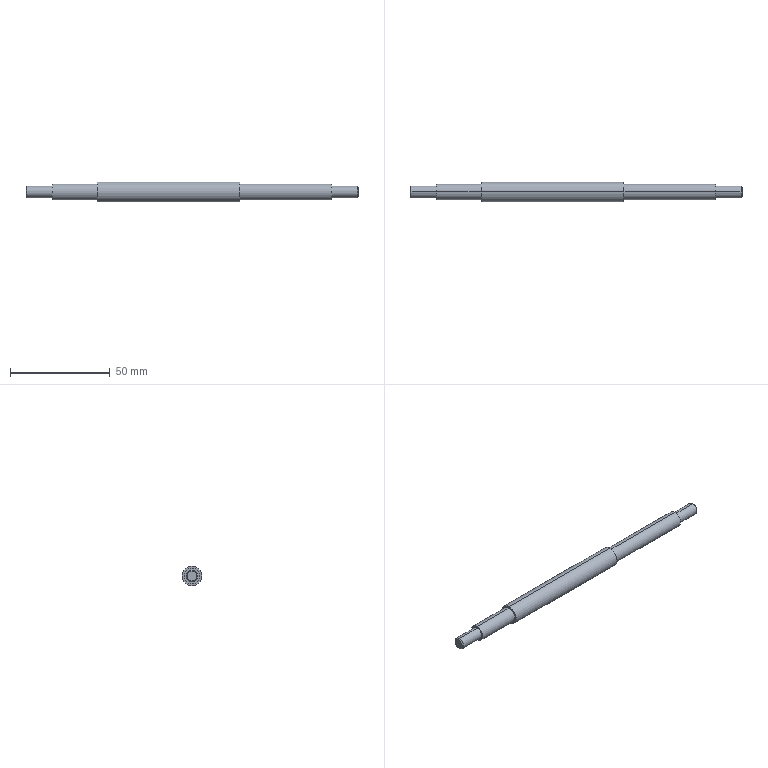Part | SolidWorks | features Revolution 1 | 1 solid | 20 faces | box 166.354 x 10 x 10 mm | volume 9800 mm3 | cylinder 10 | plane 6 | cone 4 | commonest cylinder face diameters 6 x4 8 x4 10 x2
STEP:
#1=CARTESIAN_POINT('',(-205.748,-31.205,-3.));
#2=VERTEX_POINT('',#1);
#3=CARTESIAN_POINT('',(-205.748,-31.205,3.));
#4=VERTEX_POINT('',#3);
#5=CARTESIAN_POINT('',(-205.748,-31.205,0.));
#6=DIRECTION('',(1.,0.,0.));
#7=DIRECTION('',(0.,0.,-1.));
#8=AXIS2_PLACEMENT_3D('',#5,#6,#7);
#9=CIRCLE('',#8,3.);
#10=EDGE_CURVE('',#2,#4,#9,.T.);
#11=ORIENTED_EDGE('',*,*,#10,.T.);
#12=CARTESIAN_POINT('',(-193.072,-31.205,3.));
#13=VERTEX_POINT('',#12);
#14=CARTESIAN_POINT('',(-206.248,-31.205,3.));
#15=DIRECTION('',(1.,0.,0.));
#16=VECTOR('',#15,1000.);
#17=LINE('',#14,#16);
#18=EDGE_CURVE('',#4,#13,#17,.T.);
#19=ORIENTED_EDGE('',*,*,#18,.T.);
#20=CARTESIAN_POINT('',(-193.072,-31.205,-3.));
#21=VERTEX_POINT('',#20);
#22=CARTESIAN_POINT('',(-193.072,-31.205,0.));
#23=DIRECTION('',(1.,0.,0.));
#24=DIRECTION('',(0.,0.,-1.));
#25=AXIS2_PLACEMENT_3D('',#22,#23,#24);
#26=CIRCLE('',#25,3.);
#27=EDGE_CURVE('',#21,#13,#26,.T.);
#28=ORIENTED_EDGE('',*,*,#27,.F.);
#29=CARTESIAN_POINT('',(-206.248,-31.205,-3.));
#30=DIRECTION('',(1.,0.,0.));
#31=VECTOR('',#30,1000.);
#32=LINE('',#29,#31);
#33=EDGE_CURVE('',#2,#21,#32,.T.);
#34=ORIENTED_EDGE('',*,*,#33,.F.);
#35=EDGE_LOOP('',(#11,#19,#28,#34));
#36=FACE_OUTER_BOUND('',#35,.T.);
#37=CARTESIAN_POINT('',(-206.248,-31.205,0.));
#38=DIRECTION('',(1.,0.,0.));
#39=DIRECTION('',(0.,0.,-1.));
#40=AXIS2_PLACEMENT_3D('',#37,#38,#39);
#41=CYLINDRICAL_SURFACE('',#40,3.);
#42=ADVANCED_FACE('',(#36),#41,.T.);
#43=CARTESIAN_POINT('',(-206.248,-31.205,-2.5));
#44=VERTEX_POINT('',#43);
#45=CARTESIAN_POINT('',(-206.248,-31.205,2.5));
#46=VERTEX_POINT('',#45);
#47=CARTESIAN_POINT('',(-206.248,-31.205,0.));
#48=DIRECTION('',(1.,0.,0.));
#49=DIRECTION('',(0.,0.,-1.));
#50=AXIS2_PLACEMENT_3D('',#47,#48,#49);
#51=CIRCLE('',#50,2.5);
#52=EDGE_CURVE('',#44,#46,#51,.T.);
#53=ORIENTED_EDGE('',*,*,#52,.T.);
#54=CARTESIAN_POINT('',(-205.748,-31.205,3.));
#55=DIRECTION('',(0.7071,0.,0.7071));
#56=VECTOR('',#55,1000.);
#57=LINE('',#54,#56);
#58=EDGE_CURVE('',#46,#4,#57,.T.);
#59=ORIENTED_EDGE('',*,*,#58,.T.);
#60=ORIENTED_EDGE('',*,*,#10,.F.);
#61=CARTESIAN_POINT('',(-205.748,-31.205,-3.));
#62=DIRECTION('',(0.7071,0.,-0.7071));
#63=VECTOR('',#62,1000.);
#64=LINE('',#61,#63);
#65=EDGE_CURVE('',#44,#2,#64,.T.);
#66=ORIENTED_EDGE('',*,*,#65,.F.);
#67=EDGE_LOOP('',(#53,#59,#60,#66));
#68=FACE_OUTER_BOUND('',#67,.T.);
#69=CARTESIAN_POINT('',(-205.748,-31.205,0.));
#70=DIRECTION('',(1.,0.,0.));
#71=DIRECTION('',(0.,0.,-1.));
#72=AXIS2_PLACEMENT_3D('',#69,#70,#71);
#73=CONICAL_SURFACE('',#72,3.,0.7854);
#74=ADVANCED_FACE('',(#68),#73,.T.);
#75=CARTESIAN_POINT('',(-39.895,-31.205,-2.5));
#76=VERTEX_POINT('',#75);
#77=CARTESIAN_POINT('',(-39.895,-31.205,2.5));
#78=VERTEX_POINT('',#77);
#79=CARTESIAN_POINT('',(-39.895,-31.205,0.));
#80=DIRECTION('',(1.,0.,0.));
#81=DIRECTION('',(0.,0.,-1.));
#82=AXIS2_PLACEMENT_3D('',#79,#80,#81);
#83=CIRCLE('',#82,2.5);
#84=EDGE_CURVE('',#76,#78,#83,.T.);
#85=ORIENTED_EDGE('',*,*,#84,.F.);
#86=CARTESIAN_POINT('',(-40.395,-31.205,-3.));
#87=VERTEX_POINT('',#86);
#88=CARTESIAN_POINT('',(-39.895,-31.205,-2.5));
#89=DIRECTION('',(-0.7071,0.,-0.7071));
#90=VECTOR('',#89,1000.);
#91=LINE('',#88,#90);
#92=EDGE_CURVE('',#76,#87,#91,.T.);
#93=ORIENTED_EDGE('',*,*,#92,.T.);
#94=CARTESIAN_POINT('',(-40.395,-31.205,3.));
#95=VERTEX_POINT('',#94);
#96=CARTESIAN_POINT('',(-40.395,-31.205,0.));
#97=DIRECTION('',(1.,0.,0.));
#98=DIRECTION('',(0.,0.,-1.));
#99=AXIS2_PLACEMENT_3D('',#96,#97,#98);
#100=CIRCLE('',#99,3.);
#101=EDGE_CURVE('',#87,#95,#100,.T.);
#102=ORIENTED_EDGE('',*,*,#101,.T.);
#103=CARTESIAN_POINT('',(-39.895,-31.205,2.5));
#104=DIRECTION('',(-0.7071,0.,0.7071));
#105=VECTOR('',#104,1000.);
#106=LINE('',#103,#105);
#107=EDGE_CURVE('',#78,#95,#106,.T.);
#108=ORIENTED_EDGE('',*,*,#107,.F.);
#109=EDGE_LOOP('',(#85,#93,#102,#108));
#110=FACE_OUTER_BOUND('',#109,.T.);
#111=CARTESIAN_POINT('',(-39.895,-31.205,0.));
#112=DIRECTION('',(-1.,0.,0.));
#113=DIRECTION('',(0.,0.,1.));
#114=AXIS2_PLACEMENT_3D('',#111,#112,#113);
#115=CONICAL_SURFACE('',#114,2.5,0.7854);
#116=ADVANCED_FACE('',(#110),#115,.T.);
#117=CARTESIAN_POINT('',(-53.072,-31.205,-3.));
#118=VERTEX_POINT('',#117);
#119=CARTESIAN_POINT('',(-53.072,-31.205,3.));
#120=VERTEX_POINT('',#119);
#121=CARTESIAN_POINT('',(-53.072,-31.205,0.));
#122=DIRECTION('',(1.,0.,0.));
#123=DIRECTION('',(0.,0.,-1.));
#124=AXIS2_PLACEMENT_3D('',#121,#122,#123);
#125=CIRCLE('',#124,3.);
#126=EDGE_CURVE('',#118,#120,#125,.T.);
#127=ORIENTED_EDGE('',*,*,#126,.T.);
#128=CARTESIAN_POINT('',(-206.248,-31.205,3.));
#129=DIRECTION('',(1.,0.,0.));
#130=VECTOR('',#129,1000.);
#131=LINE('',#128,#130);
#132=EDGE_CURVE('',#120,#95,#131,.T.);
#133=ORIENTED_EDGE('',*,*,#132,.T.);
#134=ORIENTED_EDGE('',*,*,#101,.F.);
#135=CARTESIAN_POINT('',(-206.248,-31.205,-3.));
#136=DIRECTION('',(1.,0.,0.));
#137=VECTOR('',#136,1000.);
#138=LINE('',#135,#137);
#139=EDGE_CURVE('',#118,#87,#138,.T.);
#140=ORIENTED_EDGE('',*,*,#139,.F.);
#141=EDGE_LOOP('',(#127,#133,#134,#140));
#142=FACE_OUTER_BOUND('',#141,.T.);
#143=CARTESIAN_POINT('',(-206.248,-31.205,0.));
#144=DIRECTION('',(1.,0.,0.));
#145=DIRECTION('',(0.,0.,-1.));
#146=AXIS2_PLACEMENT_3D('',#143,#144,#145);
#147=CYLINDRICAL_SURFACE('',#146,3.);
#148=ADVANCED_FACE('',(#142),#147,.T.);
#149=CARTESIAN_POINT('',(-99.022,-31.205,-4.));
#150=VERTEX_POINT('',#149);
#151=CARTESIAN_POINT('',(-99.022,-31.205,4.));
#152=VERTEX_POINT('',#151);
#153=CARTESIAN_POINT('',(-99.022,-31.205,0.));
#154=DIRECTION('',(1.,0.,0.));
#155=DIRECTION('',(0.,0.,-1.));
#156=AXIS2_PLACEMENT_3D('',#153,#154,#155);
#157=CIRCLE('',#156,4.);
#158=EDGE_CURVE('',#150,#152,#157,.T.);
#159=ORIENTED_EDGE('',*,*,#158,.T.);
#160=CARTESIAN_POINT('',(-53.072,-31.205,4.));
#161=VERTEX_POINT('',#160);
#162=CARTESIAN_POINT('',(-206.248,-31.205,4.));
#163=DIRECTION('',(1.,0.,0.));
#164=VECTOR('',#163,1000.);
#165=LINE('',#162,#164);
#166=EDGE_CURVE('',#152,#161,#165,.T.);
#167=ORIENTED_EDGE('',*,*,#166,.T.);
#168=CARTESIAN_POINT('',(-53.072,-31.205,-4.));
#169=VERTEX_POINT('',#168);
#170=CARTESIAN_POINT('',(-53.072,-31.205,0.));
#171=DIRECTION('',(1.,0.,0.));
#172=DIRECTION('',(0.,0.,-1.));
#173=AXIS2_PLACEMENT_3D('',#170,#171,#172);
#174=CIRCLE('',#173,4.);
#175=EDGE_CURVE('',#169,#161,#174,.T.);
#176=ORIENTED_EDGE('',*,*,#175,.F.);
#177=CARTESIAN_POINT('',(-206.248,-31.205,-4.));
#178=DIRECTION('',(1.,0.,0.));
#179=VECTOR('',#178,1000.);
#180=LINE('',#177,#179);
#181=EDGE_CURVE('',#150,#169,#180,.T.);
#182=ORIENTED_EDGE('',*,*,#181,.F.);
#183=EDGE_LOOP('',(#159,#167,#176,#182));
#184=FACE_OUTER_BOUND('',#183,.T.);
#185=CARTESIAN_POINT('',(-206.248,-31.205,0.));
#186=DIRECTION('',(1.,0.,0.));
#187=DIRECTION('',(0.,0.,-1.));
#188=AXIS2_PLACEMENT_3D('',#185,#186,#187);
#189=CYLINDRICAL_SURFACE('',#188,4.);
#190=ADVANCED_FACE('',(#184),#189,.T.);
#191=CARTESIAN_POINT('',(-170.527,-31.205,-5.));
#192=VERTEX_POINT('',#191);
#193=CARTESIAN_POINT('',(-170.527,-31.205,5.));
#194=VERTEX_POINT('',#193);
#195=CARTESIAN_POINT('',(-170.527,-31.205,0.));
#196=DIRECTION('',(1.,0.,0.));
#197=DIRECTION('',(0.,0.,-1.));
#198=AXIS2_PLACEMENT_3D('',#195,#196,#197);
#199=CIRCLE('',#198,5.);
#200=EDGE_CURVE('',#192,#194,#199,.T.);
#201=ORIENTED_EDGE('',*,*,#200,.T.);
#202=CARTESIAN_POINT('',(-99.022,-31.205,5.));
#203=VERTEX_POINT('',#202);
#204=CARTESIAN_POINT('',(-206.248,-31.205,5.));
#205=DIRECTION('',(1.,0.,0.));
#206=VECTOR('',#205,1000.);
#207=LINE('',#204,#206);
#208=EDGE_CURVE('',#194,#203,#207,.T.);
#209=ORIENTED_EDGE('',*,*,#208,.T.);
#210=CARTESIAN_POINT('',(-99.022,-31.205,-5.));
#211=VERTEX_POINT('',#210);
#212=CARTESIAN_POINT('',(-99.022,-31.205,0.));
#213=DIRECTION('',(1.,0.,0.));
#214=DIRECTION('',(0.,0.,-1.));
#215=AXIS2_PLACEMENT_3D('',#212,#213,#214);
#216=CIRCLE('',#215,5.);
#217=EDGE_CURVE('',#211,#203,#216,.T.);
#218=ORIENTED_EDGE('',*,*,#217,.F.);
#219=CARTESIAN_POINT('',(-206.248,-31.205,-5.));
#220=DIRECTION('',(1.,0.,0.));
#221=VECTOR('',#220,1000.);
#222=LINE('',#219,#221);
#223=EDGE_CURVE('',#192,#211,#222,.T.);
#224=ORIENTED_EDGE('',*,*,#223,.F.);
#225=EDGE_LOOP('',(#201,#209,#218,#224));
#226=FACE_OUTER_BOUND('',#225,.T.);
#227=CARTESIAN_POINT('',(-206.248,-31.205,0.));
#228=DIRECTION('',(1.,0.,0.));
#229=DIRECTION('',(0.,0.,-1.));
#230=AXIS2_PLACEMENT_3D('',#227,#228,#229);
#231=CYLINDRICAL_SURFACE('',#230,5.);
#232=ADVANCED_FACE('',(#226),#231,.T.);
#233=CARTESIAN_POINT('',(-193.072,-31.205,-4.));
#234=VERTEX_POINT('',#233);
#235=CARTESIAN_POINT('',(-193.072,-31.205,4.));
#236=VERTEX_POINT('',#235);
#237=CARTESIAN_POINT('',(-193.072,-31.205,0.));
#238=DIRECTION('',(1.,0.,0.));
#239=DIRECTION('',(0.,0.,-1.));
#240=AXIS2_PLACEMENT_3D('',#237,#238,#239);
#241=CIRCLE('',#240,4.);
#242=EDGE_CURVE('',#234,#236,#241,.T.);
#243=ORIENTED_EDGE('',*,*,#242,.T.);
#244=CARTESIAN_POINT('',(-170.527,-31.205,4.));
#245=VERTEX_POINT('',#244);
#246=CARTESIAN_POINT('',(-206.248,-31.205,4.));
#247=DIRECTION('',(1.,0.,0.));
#248=VECTOR('',#247,1000.);
#249=LINE('',#246,#248);
#250=EDGE_CURVE('',#236,#245,#249,.T.);
#251=ORIENTED_EDGE('',*,*,#250,.T.);
#252=CARTESIAN_POINT('',(-170.527,-31.205,-4.));
#253=VERTEX_POINT('',#252);
#254=CARTESIAN_POINT('',(-170.527,-31.205,0.));
#255=DIRECTION('',(1.,0.,0.));
#256=DIRECTION('',(0.,0.,-1.));
#257=AXIS2_PLACEMENT_3D('',#254,#255,#256);
#258=CIRCLE('',#257,4.);
#259=EDGE_CURVE('',#253,#245,#258,.T.);
#260=ORIENTED_EDGE('',*,*,#259,.F.);
#261=CARTESIAN_POINT('',(-206.248,-31.205,-4.));
#262=DIRECTION('',(1.,0.,0.));
#263=VECTOR('',#262,1000.);
#264=LINE('',#261,#263);
#265=EDGE_CURVE('',#234,#253,#264,.T.);
#266=ORIENTED_EDGE('',*,*,#265,.F.);
#267=EDGE_LOOP('',(#243,#251,#260,#266));
#268=FACE_OUTER_BOUND('',#267,.T.);
#269=CARTESIAN_POINT('',(-206.248,-31.205,0.));
#270=DIRECTION('',(1.,0.,0.));
#271=DIRECTION('',(0.,0.,-1.));
#272=AXIS2_PLACEMENT_3D('',#269,#270,#271);
#273=CYLINDRICAL_SURFACE('',#272,4.);
#274=ADVANCED_FACE('',(#268),#273,.T.);
#275=ORIENTED_EDGE('',*,*,#250,.F.);
#276=CARTESIAN_POINT('',(-193.072,-31.205,0.));
#277=DIRECTION('',(1.,0.,0.));
#278=DIRECTION('',(0.,0.,-1.));
#279=AXIS2_PLACEMENT_3D('',#276,#277,#278);
#280=CIRCLE('',#279,4.);
#281=EDGE_CURVE('',#236,#234,#280,.T.);
#282=ORIENTED_EDGE('',*,*,#281,.T.);
#283=ORIENTED_EDGE('',*,*,#265,.T.);
#284=CARTESIAN_POINT('',(-170.527,-31.205,0.));
#285=DIRECTION('',(1.,0.,0.));
#286=DIRECTION('',(0.,0.,-1.));
#287=AXIS2_PLACEMENT_3D('',#284,#285,#286);
#288=CIRCLE('',#287,4.);
#289=EDGE_CURVE('',#245,#253,#288,.T.);
#290=ORIENTED_EDGE('',*,*,#289,.F.);
#291=EDGE_LOOP('',(#275,#282,#283,#290));
#292=FACE_OUTER_BOUND('',#291,.T.);
#293=CARTESIAN_POINT('',(-206.248,-31.205,0.));
#294=DIRECTION('',(1.,0.,0.));
#295=DIRECTION('',(0.,0.,-1.));
#296=AXIS2_PLACEMENT_3D('',#293,#294,#295);
#297=CYLINDRICAL_SURFACE('',#296,4.);
#298=ADVANCED_FACE('',(#292),#297,.T.);
#299=ORIENTED_EDGE('',*,*,#259,.T.);
#300=ORIENTED_EDGE('',*,*,#289,.T.);
#301=EDGE_LOOP('',(#299,#300));
#302=FACE_BOUND('',#301,.T.);
#303=ORIENTED_EDGE('',*,*,#200,.F.);
#304=CARTESIAN_POINT('',(-170.527,-31.205,0.));
#305=DIRECTION('',(1.,0.,0.));
#306=DIRECTION('',(0.,0.,-1.));
#307=AXIS2_PLACEMENT_3D('',#304,#305,#306);
#308=CIRCLE('',#307,5.);
#309=EDGE_CURVE('',#194,#192,#308,.T.);
#310=ORIENTED_EDGE('',*,*,#309,.F.);
#311=EDGE_LOOP('',(#303,#310));
#312=FACE_OUTER_BOUND('',#311,.T.);
#313=CARTESIAN_POINT('',(-170.527,-27.205,0.));
#314=DIRECTION('',(-1.,0.,0.));
#315=DIRECTION('',(0.,0.,1.));
#316=AXIS2_PLACEMENT_3D('',#313,#314,#315);
#317=PLANE('',#316);
#318=ADVANCED_FACE('',(#302,#312),#317,.T.);
#319=ORIENTED_EDGE('',*,*,#208,.F.);
#320=ORIENTED_EDGE('',*,*,#309,.T.);
#321=ORIENTED_EDGE('',*,*,#223,.T.);
#322=CARTESIAN_POINT('',(-99.022,-31.205,0.));
#323=DIRECTION('',(1.,0.,0.));
#324=DIRECTION('',(0.,0.,-1.));
#325=AXIS2_PLACEMENT_3D('',#322,#323,#324);
#326=CIRCLE('',#325,5.);
#327=EDGE_CURVE('',#203,#211,#326,.T.);
#328=ORIENTED_EDGE('',*,*,#327,.F.);
#329=EDGE_LOOP('',(#319,#320,#321,#328));
#330=FACE_OUTER_BOUND('',#329,.T.);
#331=CARTESIAN_POINT('',(-206.248,-31.205,0.));
#332=DIRECTION('',(1.,0.,0.));
#333=DIRECTION('',(0.,0.,-1.));
#334=AXIS2_PLACEMENT_3D('',#331,#332,#333);
#335=CYLINDRICAL_SURFACE('',#334,5.);
#336=ADVANCED_FACE('',(#330),#335,.T.);
#337=ORIENTED_EDGE('',*,*,#217,.T.);
#338=ORIENTED_EDGE('',*,*,#327,.T.);
#339=EDGE_LOOP('',(#337,#338));
#340=FACE_OUTER_BOUND('',#339,.T.);
#341=ORIENTED_EDGE('',*,*,#158,.F.);
#342=CARTESIAN_POINT('',(-99.022,-31.205,0.));
#343=DIRECTION('',(1.,0.,0.));
#344=DIRECTION('',(0.,0.,-1.));
#345=AXIS2_PLACEMENT_3D('',#342,#343,#344);
#346=CIRCLE('',#345,4.);
#347=EDGE_CURVE('',#152,#150,#346,.T.);
#348=ORIENTED_EDGE('',*,*,#347,.F.);
#349=EDGE_LOOP('',(#341,#348));
#350=FACE_BOUND('',#349,.T.);
#351=CARTESIAN_POINT('',(-99.022,-26.205,0.));
#352=DIRECTION('',(1.,0.,0.));
#353=DIRECTION('',(0.,0.,-1.));
#354=AXIS2_PLACEMENT_3D('',#351,#352,#353);
#355=PLANE('',#354);
#356=ADVANCED_FACE('',(#340,#350),#355,.T.);
#357=ORIENTED_EDGE('',*,*,#166,.F.);
#358=ORIENTED_EDGE('',*,*,#347,.T.);
#359=ORIENTED_EDGE('',*,*,#181,.T.);
#360=CARTESIAN_POINT('',(-53.072,-31.205,0.));
#361=DIRECTION('',(1.,0.,0.));
#362=DIRECTION('',(0.,0.,-1.));
#363=AXIS2_PLACEMENT_3D('',#360,#361,#362);
#364=CIRCLE('',#363,4.);
#365=EDGE_CURVE('',#161,#169,#364,.T.);
#366=ORIENTED_EDGE('',*,*,#365,.F.);
#367=EDGE_LOOP('',(#357,#358,#359,#366));
#368=FACE_OUTER_BOUND('',#367,.T.);
#369=CARTESIAN_POINT('',(-206.248,-31.205,0.));
#370=DIRECTION('',(1.,0.,0.));
#371=DIRECTION('',(0.,0.,-1.));
#372=AXIS2_PLACEMENT_3D('',#369,#370,#371);
#373=CYLINDRICAL_SURFACE('',#372,4.);
#374=ADVANCED_FACE('',(#368),#373,.T.);
#375=ORIENTED_EDGE('',*,*,#175,.T.);
#376=ORIENTED_EDGE('',*,*,#365,.T.);
#377=EDGE_LOOP('',(#375,#376));
#378=FACE_OUTER_BOUND('',#377,.T.);
#379=ORIENTED_EDGE('',*,*,#126,.F.);
#380=CARTESIAN_POINT('',(-53.072,-31.205,0.));
#381=DIRECTION('',(1.,0.,0.));
#382=DIRECTION('',(0.,0.,-1.));
#383=AXIS2_PLACEMENT_3D('',#380,#381,#382);
#384=CIRCLE('',#383,3.);
#385=EDGE_CURVE('',#120,#118,#384,.T.);
#386=ORIENTED_EDGE('',*,*,#385,.F.);
#387=EDGE_LOOP('',(#379,#386));
#388=FACE_BOUND('',#387,.T.);
#389=CARTESIAN_POINT('',(-53.072,-28.205,0.));
#390=DIRECTION('',(1.,0.,0.));
#391=DIRECTION('',(0.,0.,-1.));
#392=AXIS2_PLACEMENT_3D('',#389,#390,#391);
#393=PLANE('',#392);
#394=ADVANCED_FACE('',(#378,#388),#393,.T.);
#395=ORIENTED_EDGE('',*,*,#132,.F.);
#396=ORIENTED_EDGE('',*,*,#385,.T.);
#397=ORIENTED_EDGE('',*,*,#139,.T.);
#398=CARTESIAN_POINT('',(-40.395,-31.205,0.));
#399=DIRECTION('',(1.,0.,0.));
#400=DIRECTION('',(0.,0.,-1.));
#401=AXIS2_PLACEMENT_3D('',#398,#399,#400);
#402=CIRCLE('',#401,3.);
#403=EDGE_CURVE('',#95,#87,#402,.T.);
#404=ORIENTED_EDGE('',*,*,#403,.F.);
#405=EDGE_LOOP('',(#395,#396,#397,#404));
#406=FACE_OUTER_BOUND('',#405,.T.);
#407=CARTESIAN_POINT('',(-206.248,-31.205,0.));
#408=DIRECTION('',(1.,0.,0.));
#409=DIRECTION('',(0.,0.,-1.));
#410=AXIS2_PLACEMENT_3D('',#407,#408,#409);
#411=CYLINDRICAL_SURFACE('',#410,3.);
#412=ADVANCED_FACE('',(#406),#411,.T.);
#413=ORIENTED_EDGE('',*,*,#92,.F.);
#414=CARTESIAN_POINT('',(-39.895,-31.205,0.));
#415=DIRECTION('',(1.,0.,0.));
#416=DIRECTION('',(0.,0.,-1.));
#417=AXIS2_PLACEMENT_3D('',#414,#415,#416);
#418=CIRCLE('',#417,2.5);
#419=EDGE_CURVE('',#78,#76,#418,.T.);
#420=ORIENTED_EDGE('',*,*,#419,.F.);
#421=ORIENTED_EDGE('',*,*,#107,.T.);
#422=ORIENTED_EDGE('',*,*,#403,.T.);
#423=EDGE_LOOP('',(#413,#420,#421,#422));
#424=FACE_OUTER_BOUND('',#423,.T.);
#425=CARTESIAN_POINT('',(-39.895,-31.205,0.));
#426=DIRECTION('',(-1.,0.,0.));
#427=DIRECTION('',(0.,0.,1.));
#428=AXIS2_PLACEMENT_3D('',#425,#426,#427);
#429=CONICAL_SURFACE('',#428,2.5,0.7854);
#430=ADVANCED_FACE('',(#424),#429,.T.);
#431=ORIENTED_EDGE('',*,*,#419,.T.);
#432=ORIENTED_EDGE('',*,*,#84,.T.);
#433=EDGE_LOOP('',(#431,#432));
#434=FACE_OUTER_BOUND('',#433,.T.);
#435=CARTESIAN_POINT('',(-39.895,-28.705,0.));
#436=DIRECTION('',(1.,0.,0.));
#437=DIRECTION('',(0.,0.,-1.));
#438=AXIS2_PLACEMENT_3D('',#435,#436,#437);
#439=PLANE('',#438);
#440=ADVANCED_FACE('',(#434),#439,.T.);
#441=ORIENTED_EDGE('',*,*,#52,.F.);
#442=CARTESIAN_POINT('',(-206.248,-31.205,0.));
#443=DIRECTION('',(1.,0.,0.));
#444=DIRECTION('',(0.,0.,-1.));
#445=AXIS2_PLACEMENT_3D('',#442,#443,#444);
#446=CIRCLE('',#445,2.5);
#447=EDGE_CURVE('',#46,#44,#446,.T.);
#448=ORIENTED_EDGE('',*,*,#447,.F.);
#449=EDGE_LOOP('',(#441,#448));
#450=FACE_OUTER_BOUND('',#449,.T.);
#451=CARTESIAN_POINT('',(-206.248,-28.705,0.));
#452=DIRECTION('',(-1.,0.,0.));
#453=DIRECTION('',(0.,0.,1.));
#454=AXIS2_PLACEMENT_3D('',#451,#452,#453);
#455=PLANE('',#454);
#456=ADVANCED_FACE('',(#450),#455,.T.);
#457=ORIENTED_EDGE('',*,*,#58,.F.);
#458=ORIENTED_EDGE('',*,*,#447,.T.);
#459=ORIENTED_EDGE('',*,*,#65,.T.);
#460=CARTESIAN_POINT('',(-205.748,-31.205,0.));
#461=DIRECTION('',(1.,0.,0.));
#462=DIRECTION('',(0.,0.,-1.));
#463=AXIS2_PLACEMENT_3D('',#460,#461,#462);
#464=CIRCLE('',#463,3.);
#465=EDGE_CURVE('',#4,#2,#464,.T.);
#466=ORIENTED_EDGE('',*,*,#465,.F.);
#467=EDGE_LOOP('',(#457,#458,#459,#466));
#468=FACE_OUTER_BOUND('',#467,.T.);
#469=CARTESIAN_POINT('',(-205.748,-31.205,0.));
#470=DIRECTION('',(1.,0.,0.));
#471=DIRECTION('',(0.,0.,-1.));
#472=AXIS2_PLACEMENT_3D('',#469,#470,#471);
#473=CONICAL_SURFACE('',#472,3.,0.7854);
#474=ADVANCED_FACE('',(#468),#473,.T.);
#475=ORIENTED_EDGE('',*,*,#18,.F.);
#476=ORIENTED_EDGE('',*,*,#465,.T.);
#477=ORIENTED_EDGE('',*,*,#33,.T.);
#478=CARTESIAN_POINT('',(-193.072,-31.205,0.));
#479=DIRECTION('',(1.,0.,0.));
#480=DIRECTION('',(0.,0.,-1.));
#481=AXIS2_PLACEMENT_3D('',#478,#479,#480);
#482=CIRCLE('',#481,3.);
#483=EDGE_CURVE('',#13,#21,#482,.T.);
#484=ORIENTED_EDGE('',*,*,#483,.F.);
#485=EDGE_LOOP('',(#475,#476,#477,#484));
#486=FACE_OUTER_BOUND('',#485,.T.);
#487=CARTESIAN_POINT('',(-206.248,-31.205,0.));
#488=DIRECTION('',(1.,0.,0.));
#489=DIRECTION('',(0.,0.,-1.));
#490=AXIS2_PLACEMENT_3D('',#487,#488,#489);
#491=CYLINDRICAL_SURFACE('',#490,3.);
#492=ADVANCED_FACE('',(#486),#491,.T.);
#493=ORIENTED_EDGE('',*,*,#27,.T.);
#494=ORIENTED_EDGE('',*,*,#483,.T.);
#495=EDGE_LOOP('',(#493,#494));
#496=FACE_BOUND('',#495,.T.);
#497=ORIENTED_EDGE('',*,*,#242,.F.);
#498=ORIENTED_EDGE('',*,*,#281,.F.);
#499=EDGE_LOOP('',(#497,#498));
#500=FACE_OUTER_BOUND('',#499,.T.);
#501=CARTESIAN_POINT('',(-193.072,-28.205,0.));
#502=DIRECTION('',(-1.,0.,0.));
#503=DIRECTION('',(0.,0.,1.));
#504=AXIS2_PLACEMENT_3D('',#501,#502,#503);
#505=PLANE('',#504);
#506=ADVANCED_FACE('',(#496,#500),#505,.T.);
#507=CLOSED_SHELL('',(#42,#74,#116,#148,#190,#232,#274,#298,#318,#336,#356,#374,#394,#412,#430,#440,#456,#474,#492,#506));
#508=MANIFOLD_SOLID_BREP('',#507);
#509=CARTESIAN_POINT('',(0.,0.,0.));
#510=DIRECTION('',(0.,0.,1.));
#511=DIRECTION('',(1.,0.,0.));
#512=AXIS2_PLACEMENT_3D('',#509,#510,#511);
#513=(LENGTH_UNIT()NAMED_UNIT(*)SI_UNIT(.MILLI.,.METRE.));
#514=UNCERTAINTY_MEASURE_WITH_UNIT(LENGTH_MEASURE(0.00001),#513,'','');
#515=(NAMED_UNIT(*)PLANE_ANGLE_UNIT()SI_UNIT($,.RADIAN.));
#516=(NAMED_UNIT(*)SI_UNIT($,.STERADIAN.)SOLID_ANGLE_UNIT());
#517=(GEOMETRIC_REPRESENTATION_CONTEXT(3)GLOBAL_UNCERTAINTY_ASSIGNED_CONTEXT((#514))GLOBAL_UNIT_ASSIGNED_CONTEXT((#513,#515,#516))REPRESENTATION_CONTEXT('',''));
#518=ADVANCED_BREP_SHAPE_REPRESENTATION('',(#508,#512),#517);